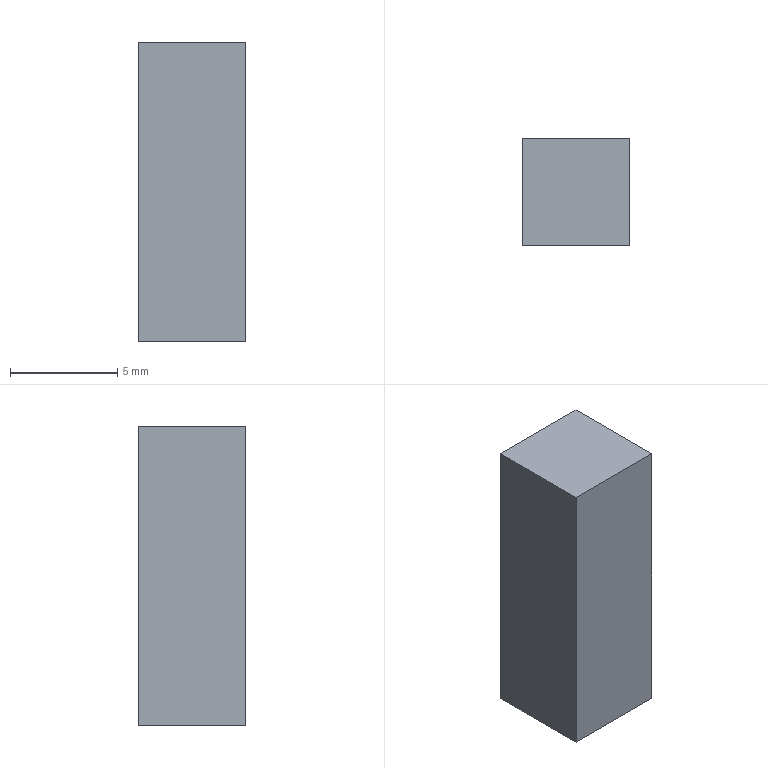Part | STEP file | 1 solid | 6 faces | box 5 x 5 x 14 mm | volume 350 mm3 | plane 6
STEP:
#1=CARTESIAN_POINT('',(0.,0.,0.));
#2=DIRECTION('',(0.,0.,1.));
#3=DIRECTION('',(1.,0.,0.));
#4=AXIS2_PLACEMENT_3D('',#1,#2,#3);
#5=CARTESIAN_POINT('',(-2.5,2.5,0.));
#6=VERTEX_POINT('',#5);
#7=CARTESIAN_POINT('',(-2.5,2.5,-14.));
#8=VERTEX_POINT('',#7);
#9=CARTESIAN_POINT('',(-2.5,2.5,0.));
#10=DIRECTION('',(0.,0.,-1.));
#11=VECTOR('',#10,1.);
#12=LINE('',#9,#11);
#13=CARTESIAN_POINT('',(-2.5,2.5,0.));
#14=DIRECTION('',(-1.,0.,0.));
#15=DIRECTION('',(0.,0.,1.));
#16=AXIS2_PLACEMENT_3D('',#13,#14,#15);
#17=PLANE('',#16);
#18=CARTESIAN_POINT('',(0.,0.));
#19=DIRECTION('',(-1.,0.));
#20=VECTOR('',#19,1.);
#21=LINE('',#18,#20);
#22=(GEOMETRIC_REPRESENTATION_CONTEXT(2)PARAMETRIC_REPRESENTATION_CONTEXT()REPRESENTATION_CONTEXT('',''));
#23=DEFINITIONAL_REPRESENTATION('',(#21),#22);
#24=PCURVE('',#17,#23);
#25=CARTESIAN_POINT('',(2.5,2.5,0.));
#26=DIRECTION('',(0.,1.,0.));
#27=DIRECTION('',(0.,0.,1.));
#28=AXIS2_PLACEMENT_3D('',#25,#26,#27);
#29=PLANE('',#28);
#30=CARTESIAN_POINT('',(0.,-5.));
#31=DIRECTION('',(-1.,0.));
#32=VECTOR('',#31,1.);
#33=LINE('',#30,#32);
#34=(GEOMETRIC_REPRESENTATION_CONTEXT(2)PARAMETRIC_REPRESENTATION_CONTEXT()REPRESENTATION_CONTEXT('',''));
#35=DEFINITIONAL_REPRESENTATION('',(#33),#34);
#36=PCURVE('',#29,#35);
#37=SURFACE_CURVE('',#12,(#24,#36),.PCURVE_S1.);
#38=EDGE_CURVE('',#6,#8,#37,.T.);
#39=ORIENTED_EDGE('',*,*,#38,.T.);
#40=CARTESIAN_POINT('',(-2.5,-2.5,-14.));
#41=VERTEX_POINT('',#40);
#42=CARTESIAN_POINT('',(-2.5,2.5,-14.));
#43=DIRECTION('',(0.,-1.,0.));
#44=VECTOR('',#43,1.);
#45=LINE('',#42,#44);
#46=CARTESIAN_POINT('',(-14.,0.));
#47=DIRECTION('',(0.,-1.));
#48=VECTOR('',#47,1.);
#49=LINE('',#46,#48);
#50=(GEOMETRIC_REPRESENTATION_CONTEXT(2)PARAMETRIC_REPRESENTATION_CONTEXT()REPRESENTATION_CONTEXT('',''));
#51=DEFINITIONAL_REPRESENTATION('',(#49),#50);
#52=PCURVE('',#17,#51);
#53=CARTESIAN_POINT('',(0.,0.,-14.));
#54=DIRECTION('',(0.,0.,1.));
#55=DIRECTION('',(1.,0.,0.));
#56=AXIS2_PLACEMENT_3D('',#53,#54,#55);
#57=PLANE('',#56);
#58=CARTESIAN_POINT('',(-2.5,2.5));
#59=DIRECTION('',(0.,-1.));
#60=VECTOR('',#59,1.);
#61=LINE('',#58,#60);
#62=(GEOMETRIC_REPRESENTATION_CONTEXT(2)PARAMETRIC_REPRESENTATION_CONTEXT()REPRESENTATION_CONTEXT('',''));
#63=DEFINITIONAL_REPRESENTATION('',(#61),#62);
#64=PCURVE('',#57,#63);
#65=SURFACE_CURVE('',#45,(#52,#64),.PCURVE_S1.);
#66=EDGE_CURVE('',#8,#41,#65,.T.);
#67=ORIENTED_EDGE('',*,*,#66,.T.);
#68=CARTESIAN_POINT('',(-2.5,-2.5,0.));
#69=VERTEX_POINT('',#68);
#70=CARTESIAN_POINT('',(-2.5,-2.5,0.));
#71=DIRECTION('',(0.,0.,1.));
#72=VECTOR('',#71,1.);
#73=LINE('',#70,#72);
#74=CARTESIAN_POINT('',(0.,-5.));
#75=DIRECTION('',(1.,0.));
#76=VECTOR('',#75,1.);
#77=LINE('',#74,#76);
#78=(GEOMETRIC_REPRESENTATION_CONTEXT(2)PARAMETRIC_REPRESENTATION_CONTEXT()REPRESENTATION_CONTEXT('',''));
#79=DEFINITIONAL_REPRESENTATION('',(#77),#78);
#80=PCURVE('',#17,#79);
#81=CARTESIAN_POINT('',(-2.5,-2.5,0.));
#82=DIRECTION('',(0.,-1.,0.));
#83=DIRECTION('',(0.,0.,-1.));
#84=AXIS2_PLACEMENT_3D('',#81,#82,#83);
#85=PLANE('',#84);
#86=CARTESIAN_POINT('',(0.,0.));
#87=DIRECTION('',(-1.,0.));
#88=VECTOR('',#87,1.);
#89=LINE('',#86,#88);
#90=(GEOMETRIC_REPRESENTATION_CONTEXT(2)PARAMETRIC_REPRESENTATION_CONTEXT()REPRESENTATION_CONTEXT('',''));
#91=DEFINITIONAL_REPRESENTATION('',(#89),#90);
#92=PCURVE('',#85,#91);
#93=SURFACE_CURVE('',#73,(#80,#92),.PCURVE_S1.);
#94=EDGE_CURVE('',#41,#69,#93,.T.);
#95=ORIENTED_EDGE('',*,*,#94,.T.);
#96=CARTESIAN_POINT('',(-2.5,2.5,0.));
#97=DIRECTION('',(0.,1.,0.));
#98=VECTOR('',#97,1.);
#99=LINE('',#96,#98);
#100=CARTESIAN_POINT('',(0.,0.));
#101=DIRECTION('',(0.,1.));
#102=VECTOR('',#101,1.);
#103=LINE('',#100,#102);
#104=(GEOMETRIC_REPRESENTATION_CONTEXT(2)PARAMETRIC_REPRESENTATION_CONTEXT()REPRESENTATION_CONTEXT('',''));
#105=DEFINITIONAL_REPRESENTATION('',(#103),#104);
#106=PCURVE('',#17,#105);
#107=CARTESIAN_POINT('',(0.,0.,0.));
#108=DIRECTION('',(0.,0.,1.));
#109=DIRECTION('',(1.,0.,0.));
#110=AXIS2_PLACEMENT_3D('',#107,#108,#109);
#111=PLANE('',#110);
#112=CARTESIAN_POINT('',(-2.5,2.5));
#113=DIRECTION('',(0.,1.));
#114=VECTOR('',#113,1.);
#115=LINE('',#112,#114);
#116=(GEOMETRIC_REPRESENTATION_CONTEXT(2)PARAMETRIC_REPRESENTATION_CONTEXT()REPRESENTATION_CONTEXT('',''));
#117=DEFINITIONAL_REPRESENTATION('',(#115),#116);
#118=PCURVE('',#111,#117);
#119=SURFACE_CURVE('',#99,(#106,#118),.PCURVE_S1.);
#120=EDGE_CURVE('',#69,#6,#119,.T.);
#121=ORIENTED_EDGE('',*,*,#120,.T.);
#122=EDGE_LOOP('',(#39,#67,#95,#121));
#123=FACE_BOUND('',#122,.T.);
#124=ADVANCED_FACE('',(#123),#17,.T.);
#125=CARTESIAN_POINT('',(2.5,-2.5,-14.));
#126=VERTEX_POINT('',#125);
#127=CARTESIAN_POINT('',(0.,-2.5,-14.));
#128=DIRECTION('',(1.,0.,0.));
#129=VECTOR('',#128,1.);
#130=LINE('',#127,#129);
#131=CARTESIAN_POINT('',(0.,-2.5));
#132=DIRECTION('',(1.,0.));
#133=VECTOR('',#132,1.);
#134=LINE('',#131,#133);
#135=(GEOMETRIC_REPRESENTATION_CONTEXT(2)PARAMETRIC_REPRESENTATION_CONTEXT()REPRESENTATION_CONTEXT('',''));
#136=DEFINITIONAL_REPRESENTATION('',(#134),#135);
#137=PCURVE('',#57,#136);
#138=CARTESIAN_POINT('',(14.,2.5));
#139=DIRECTION('',(0.,1.));
#140=VECTOR('',#139,1.);
#141=LINE('',#138,#140);
#142=(GEOMETRIC_REPRESENTATION_CONTEXT(2)PARAMETRIC_REPRESENTATION_CONTEXT()REPRESENTATION_CONTEXT('',''));
#143=DEFINITIONAL_REPRESENTATION('',(#141),#142);
#144=PCURVE('',#85,#143);
#145=SURFACE_CURVE('',#130,(#137,#144),.PCURVE_S1.);
#146=EDGE_CURVE('',#41,#126,#145,.T.);
#147=ORIENTED_EDGE('',*,*,#146,.F.);
#148=ORIENTED_EDGE('',*,*,#66,.F.);
#149=CARTESIAN_POINT('',(2.5,2.5,-14.));
#150=VERTEX_POINT('',#149);
#151=CARTESIAN_POINT('',(0.,2.5,-14.));
#152=DIRECTION('',(-1.,0.,0.));
#153=VECTOR('',#152,1.);
#154=LINE('',#151,#153);
#155=CARTESIAN_POINT('',(0.,2.5));
#156=DIRECTION('',(-1.,0.));
#157=VECTOR('',#156,1.);
#158=LINE('',#155,#157);
#159=(GEOMETRIC_REPRESENTATION_CONTEXT(2)PARAMETRIC_REPRESENTATION_CONTEXT()REPRESENTATION_CONTEXT('',''));
#160=DEFINITIONAL_REPRESENTATION('',(#158),#159);
#161=PCURVE('',#57,#160);
#162=CARTESIAN_POINT('',(-14.,-2.5));
#163=DIRECTION('',(0.,-1.));
#164=VECTOR('',#163,1.);
#165=LINE('',#162,#164);
#166=(GEOMETRIC_REPRESENTATION_CONTEXT(2)PARAMETRIC_REPRESENTATION_CONTEXT()REPRESENTATION_CONTEXT('',''));
#167=DEFINITIONAL_REPRESENTATION('',(#165),#166);
#168=PCURVE('',#29,#167);
#169=SURFACE_CURVE('',#154,(#161,#168),.PCURVE_S1.);
#170=EDGE_CURVE('',#150,#8,#169,.T.);
#171=ORIENTED_EDGE('',*,*,#170,.F.);
#172=CARTESIAN_POINT('',(2.5,0.,-14.));
#173=DIRECTION('',(0.,1.,0.));
#174=VECTOR('',#173,1.);
#175=LINE('',#172,#174);
#176=CARTESIAN_POINT('',(2.5,0.));
#177=DIRECTION('',(0.,1.));
#178=VECTOR('',#177,1.);
#179=LINE('',#176,#178);
#180=(GEOMETRIC_REPRESENTATION_CONTEXT(2)PARAMETRIC_REPRESENTATION_CONTEXT()REPRESENTATION_CONTEXT('',''));
#181=DEFINITIONAL_REPRESENTATION('',(#179),#180);
#182=PCURVE('',#57,#181);
#183=CARTESIAN_POINT('',(2.5,-2.5,0.));
#184=DIRECTION('',(1.,0.,0.));
#185=DIRECTION('',(0.,0.,-1.));
#186=AXIS2_PLACEMENT_3D('',#183,#184,#185);
#187=PLANE('',#186);
#188=CARTESIAN_POINT('',(14.,2.5));
#189=DIRECTION('',(0.,1.));
#190=VECTOR('',#189,1.);
#191=LINE('',#188,#190);
#192=(GEOMETRIC_REPRESENTATION_CONTEXT(2)PARAMETRIC_REPRESENTATION_CONTEXT()REPRESENTATION_CONTEXT('',''));
#193=DEFINITIONAL_REPRESENTATION('',(#191),#192);
#194=PCURVE('',#187,#193);
#195=SURFACE_CURVE('',#175,(#182,#194),.PCURVE_S1.);
#196=EDGE_CURVE('',#126,#150,#195,.T.);
#197=ORIENTED_EDGE('',*,*,#196,.F.);
#198=EDGE_LOOP('',(#147,#148,#171,#197));
#199=FACE_BOUND('',#198,.T.);
#200=ADVANCED_FACE('',(#199),#57,.F.);
#201=CARTESIAN_POINT('',(2.5,2.5,0.));
#202=VERTEX_POINT('',#201);
#203=CARTESIAN_POINT('',(2.5,2.5,0.));
#204=DIRECTION('',(0.,0.,-1.));
#205=VECTOR('',#204,1.);
#206=LINE('',#203,#205);
#207=CARTESIAN_POINT('',(0.,0.));
#208=DIRECTION('',(-1.,0.));
#209=VECTOR('',#208,1.);
#210=LINE('',#207,#209);
#211=(GEOMETRIC_REPRESENTATION_CONTEXT(2)PARAMETRIC_REPRESENTATION_CONTEXT()REPRESENTATION_CONTEXT('',''));
#212=DEFINITIONAL_REPRESENTATION('',(#210),#211);
#213=PCURVE('',#29,#212);
#214=CARTESIAN_POINT('',(0.,5.));
#215=DIRECTION('',(1.,0.));
#216=VECTOR('',#215,1.);
#217=LINE('',#214,#216);
#218=(GEOMETRIC_REPRESENTATION_CONTEXT(2)PARAMETRIC_REPRESENTATION_CONTEXT()REPRESENTATION_CONTEXT('',''));
#219=DEFINITIONAL_REPRESENTATION('',(#217),#218);
#220=PCURVE('',#187,#219);
#221=SURFACE_CURVE('',#206,(#213,#220),.PCURVE_S1.);
#222=EDGE_CURVE('',#202,#150,#221,.T.);
#223=ORIENTED_EDGE('',*,*,#222,.T.);
#224=ORIENTED_EDGE('',*,*,#170,.T.);
#225=ORIENTED_EDGE('',*,*,#38,.F.);
#226=CARTESIAN_POINT('',(2.5,2.5,0.));
#227=DIRECTION('',(1.,0.,0.));
#228=VECTOR('',#227,1.);
#229=LINE('',#226,#228);
#230=CARTESIAN_POINT('',(0.,0.));
#231=DIRECTION('',(0.,1.));
#232=VECTOR('',#231,1.);
#233=LINE('',#230,#232);
#234=(GEOMETRIC_REPRESENTATION_CONTEXT(2)PARAMETRIC_REPRESENTATION_CONTEXT()REPRESENTATION_CONTEXT('',''));
#235=DEFINITIONAL_REPRESENTATION('',(#233),#234);
#236=PCURVE('',#29,#235);
#237=CARTESIAN_POINT('',(2.5,2.5));
#238=DIRECTION('',(1.,0.));
#239=VECTOR('',#238,1.);
#240=LINE('',#237,#239);
#241=(GEOMETRIC_REPRESENTATION_CONTEXT(2)PARAMETRIC_REPRESENTATION_CONTEXT()REPRESENTATION_CONTEXT('',''));
#242=DEFINITIONAL_REPRESENTATION('',(#240),#241);
#243=PCURVE('',#111,#242);
#244=SURFACE_CURVE('',#229,(#236,#243),.PCURVE_S1.);
#245=EDGE_CURVE('',#6,#202,#244,.T.);
#246=ORIENTED_EDGE('',*,*,#245,.T.);
#247=EDGE_LOOP('',(#223,#224,#225,#246));
#248=FACE_BOUND('',#247,.T.);
#249=ADVANCED_FACE('',(#248),#29,.T.);
#250=CARTESIAN_POINT('',(2.5,-2.5,0.));
#251=VERTEX_POINT('',#250);
#252=CARTESIAN_POINT('',(0.,-2.5,0.));
#253=DIRECTION('',(1.,0.,0.));
#254=VECTOR('',#253,1.);
#255=LINE('',#252,#254);
#256=CARTESIAN_POINT('',(0.,-2.5));
#257=DIRECTION('',(1.,0.));
#258=VECTOR('',#257,1.);
#259=LINE('',#256,#258);
#260=(GEOMETRIC_REPRESENTATION_CONTEXT(2)PARAMETRIC_REPRESENTATION_CONTEXT()REPRESENTATION_CONTEXT('',''));
#261=DEFINITIONAL_REPRESENTATION('',(#259),#260);
#262=PCURVE('',#111,#261);
#263=CARTESIAN_POINT('',(0.,2.5));
#264=DIRECTION('',(0.,1.));
#265=VECTOR('',#264,1.);
#266=LINE('',#263,#265);
#267=(GEOMETRIC_REPRESENTATION_CONTEXT(2)PARAMETRIC_REPRESENTATION_CONTEXT()REPRESENTATION_CONTEXT('',''));
#268=DEFINITIONAL_REPRESENTATION('',(#266),#267);
#269=PCURVE('',#85,#268);
#270=SURFACE_CURVE('',#255,(#262,#269),.PCURVE_S1.);
#271=EDGE_CURVE('',#69,#251,#270,.T.);
#272=ORIENTED_EDGE('',*,*,#271,.T.);
#273=CARTESIAN_POINT('',(2.5,0.,0.));
#274=DIRECTION('',(0.,1.,0.));
#275=VECTOR('',#274,1.);
#276=LINE('',#273,#275);
#277=CARTESIAN_POINT('',(2.5,0.));
#278=DIRECTION('',(0.,1.));
#279=VECTOR('',#278,1.);
#280=LINE('',#277,#279);
#281=(GEOMETRIC_REPRESENTATION_CONTEXT(2)PARAMETRIC_REPRESENTATION_CONTEXT()REPRESENTATION_CONTEXT('',''));
#282=DEFINITIONAL_REPRESENTATION('',(#280),#281);
#283=PCURVE('',#111,#282);
#284=CARTESIAN_POINT('',(0.,2.5));
#285=DIRECTION('',(0.,1.));
#286=VECTOR('',#285,1.);
#287=LINE('',#284,#286);
#288=(GEOMETRIC_REPRESENTATION_CONTEXT(2)PARAMETRIC_REPRESENTATION_CONTEXT()REPRESENTATION_CONTEXT('',''));
#289=DEFINITIONAL_REPRESENTATION('',(#287),#288);
#290=PCURVE('',#187,#289);
#291=SURFACE_CURVE('',#276,(#283,#290),.PCURVE_S1.);
#292=EDGE_CURVE('',#251,#202,#291,.T.);
#293=ORIENTED_EDGE('',*,*,#292,.T.);
#294=ORIENTED_EDGE('',*,*,#245,.F.);
#295=ORIENTED_EDGE('',*,*,#120,.F.);
#296=EDGE_LOOP('',(#272,#293,#294,#295));
#297=FACE_BOUND('',#296,.T.);
#298=ADVANCED_FACE('',(#297),#111,.T.);
#299=ORIENTED_EDGE('',*,*,#94,.F.);
#300=ORIENTED_EDGE('',*,*,#146,.T.);
#301=CARTESIAN_POINT('',(2.5,-2.5,0.));
#302=DIRECTION('',(0.,0.,1.));
#303=VECTOR('',#302,1.);
#304=LINE('',#301,#303);
#305=CARTESIAN_POINT('',(0.,5.));
#306=DIRECTION('',(-1.,0.));
#307=VECTOR('',#306,1.);
#308=LINE('',#305,#307);
#309=(GEOMETRIC_REPRESENTATION_CONTEXT(2)PARAMETRIC_REPRESENTATION_CONTEXT()REPRESENTATION_CONTEXT('',''));
#310=DEFINITIONAL_REPRESENTATION('',(#308),#309);
#311=PCURVE('',#85,#310);
#312=CARTESIAN_POINT('',(0.,0.));
#313=DIRECTION('',(-1.,0.));
#314=VECTOR('',#313,1.);
#315=LINE('',#312,#314);
#316=(GEOMETRIC_REPRESENTATION_CONTEXT(2)PARAMETRIC_REPRESENTATION_CONTEXT()REPRESENTATION_CONTEXT('',''));
#317=DEFINITIONAL_REPRESENTATION('',(#315),#316);
#318=PCURVE('',#187,#317);
#319=SURFACE_CURVE('',#304,(#311,#318),.PCURVE_S1.);
#320=EDGE_CURVE('',#126,#251,#319,.T.);
#321=ORIENTED_EDGE('',*,*,#320,.T.);
#322=ORIENTED_EDGE('',*,*,#271,.F.);
#323=EDGE_LOOP('',(#299,#300,#321,#322));
#324=FACE_BOUND('',#323,.T.);
#325=ADVANCED_FACE('',(#324),#85,.T.);
#326=ORIENTED_EDGE('',*,*,#320,.F.);
#327=ORIENTED_EDGE('',*,*,#196,.T.);
#328=ORIENTED_EDGE('',*,*,#222,.F.);
#329=ORIENTED_EDGE('',*,*,#292,.F.);
#330=EDGE_LOOP('',(#326,#327,#328,#329));
#331=FACE_BOUND('',#330,.T.);
#332=ADVANCED_FACE('',(#331),#187,.T.);
#333=CLOSED_SHELL('',(#124,#200,#249,#298,#325,#332));
#334=MANIFOLD_SOLID_BREP('',#333);
#335=(LENGTH_UNIT()NAMED_UNIT(*)SI_UNIT(.MILLI.,.METRE.));
#336=UNCERTAINTY_MEASURE_WITH_UNIT(LENGTH_MEASURE(0.0000001),#335,'','');
#337=(NAMED_UNIT(*)PLANE_ANGLE_UNIT()SI_UNIT($,.RADIAN.));
#338=(NAMED_UNIT(*)SI_UNIT($,.STERADIAN.)SOLID_ANGLE_UNIT());
#339=(GEOMETRIC_REPRESENTATION_CONTEXT(3)GLOBAL_UNCERTAINTY_ASSIGNED_CONTEXT((#336))GLOBAL_UNIT_ASSIGNED_CONTEXT((#335,#337,#338))REPRESENTATION_CONTEXT('',''));
#340=ADVANCED_BREP_SHAPE_REPRESENTATION('',(#4,#334),#339);